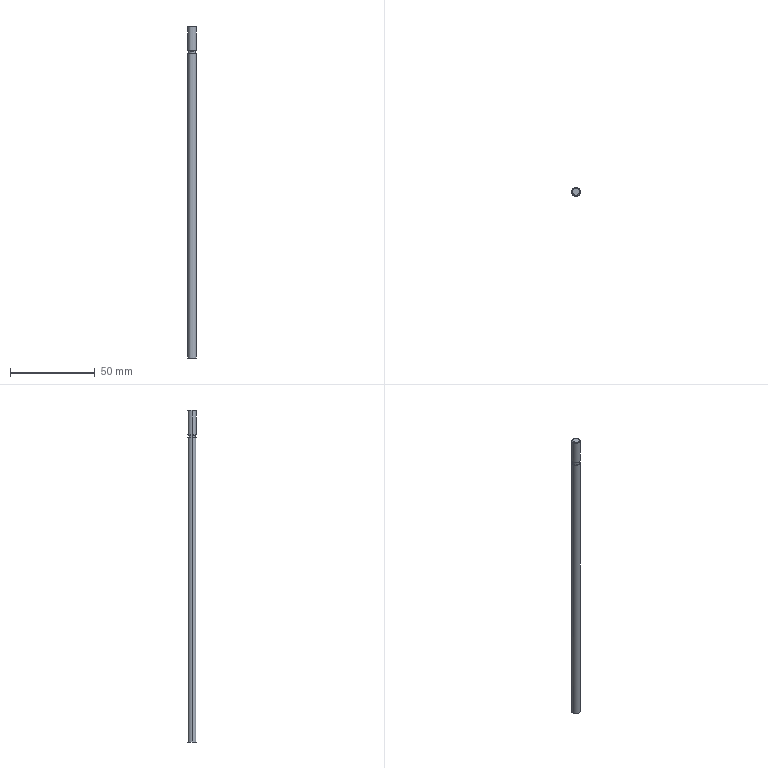Part | NX | features BREP 1 | 1 solid | 13 faces | box 5 x 5 x 196 mm | volume 3835 mm3 | cylinder 6 | cone 4 | plane 3 | commonest cylinder face diameters 5 x4 4.02 x2
STEP:
#1=CARTESIAN_POINT('',(-2.5,0.,3.5));
#2=VERTEX_POINT('',#1);
#3=CARTESIAN_POINT('',(2.5,0.,3.5));
#4=VERTEX_POINT('',#3);
#5=CARTESIAN_POINT('',(0.,0.,3.5));
#6=DIRECTION('',(0.,0.,-1.));
#7=DIRECTION('',(-1.,0.,0.));
#8=AXIS2_PLACEMENT_3D('',#5,#6,#7);
#9=CIRCLE('',#8,2.5);
#10=EDGE_CURVE('',#2,#4,#9,.T.);
#11=ORIENTED_EDGE('',*,*,#10,.T.);
#12=CARTESIAN_POINT('',(2.5,0.,-176.));
#13=VERTEX_POINT('',#12);
#14=CARTESIAN_POINT('',(2.5,0.,-86.25));
#15=DIRECTION('',(0.,0.,-1.));
#16=VECTOR('',#15,1000.);
#17=LINE('',#14,#16);
#18=EDGE_CURVE('',#4,#13,#17,.T.);
#19=ORIENTED_EDGE('',*,*,#18,.T.);
#20=CARTESIAN_POINT('',(-2.5,0.,-176.));
#21=VERTEX_POINT('',#20);
#22=CARTESIAN_POINT('',(0.,0.,-176.));
#23=DIRECTION('',(0.,0.,1.));
#24=DIRECTION('',(-1.,0.,0.));
#25=AXIS2_PLACEMENT_3D('',#22,#23,#24);
#26=CIRCLE('',#25,2.5);
#27=EDGE_CURVE('',#13,#21,#26,.T.);
#28=ORIENTED_EDGE('',*,*,#27,.T.);
#29=CARTESIAN_POINT('',(-2.5,0.,-86.25));
#30=DIRECTION('',(0.,0.,-1.));
#31=VECTOR('',#30,1000.);
#32=LINE('',#29,#31);
#33=EDGE_CURVE('',#2,#21,#32,.T.);
#34=ORIENTED_EDGE('',*,*,#33,.F.);
#35=EDGE_LOOP('',(#11,#19,#28,#34));
#36=FACE_BOUND('',#35,.T.);
#37=CARTESIAN_POINT('',(0.,0.,-86.25));
#38=DIRECTION('',(0.,0.,-1.));
#39=DIRECTION('',(-1.,0.,0.));
#40=AXIS2_PLACEMENT_3D('',#37,#38,#39);
#41=CYLINDRICAL_SURFACE('',#40,2.5);
#42=ADVANCED_FACE('',(#36),#41,.T.);
#43=CARTESIAN_POINT('',(-2.01,0.,5.));
#44=VERTEX_POINT('',#43);
#45=CARTESIAN_POINT('',(2.01,0.,5.));
#46=VERTEX_POINT('',#45);
#47=CARTESIAN_POINT('',(0.,0.,5.));
#48=DIRECTION('',(0.,0.,-1.));
#49=DIRECTION('',(-1.,0.,0.));
#50=AXIS2_PLACEMENT_3D('',#47,#48,#49);
#51=CIRCLE('',#50,2.01);
#52=EDGE_CURVE('',#44,#46,#51,.T.);
#53=ORIENTED_EDGE('',*,*,#52,.T.);
#54=CARTESIAN_POINT('',(2.01,0.,3.5));
#55=VERTEX_POINT('',#54);
#56=CARTESIAN_POINT('',(2.01,0.,4.25));
#57=DIRECTION('',(0.,0.,-1.));
#58=VECTOR('',#57,1000.);
#59=LINE('',#56,#58);
#60=EDGE_CURVE('',#46,#55,#59,.T.);
#61=ORIENTED_EDGE('',*,*,#60,.T.);
#62=CARTESIAN_POINT('',(-2.01,0.,3.5));
#63=VERTEX_POINT('',#62);
#64=CARTESIAN_POINT('',(0.,0.,3.5));
#65=DIRECTION('',(0.,0.,-1.));
#66=DIRECTION('',(-1.,0.,0.));
#67=AXIS2_PLACEMENT_3D('',#64,#65,#66);
#68=CIRCLE('',#67,2.01);
#69=EDGE_CURVE('',#63,#55,#68,.T.);
#70=ORIENTED_EDGE('',*,*,#69,.F.);
#71=CARTESIAN_POINT('',(-2.01,0.,4.25));
#72=DIRECTION('',(0.,0.,-1.));
#73=VECTOR('',#72,1000.);
#74=LINE('',#71,#73);
#75=EDGE_CURVE('',#44,#63,#74,.T.);
#76=ORIENTED_EDGE('',*,*,#75,.F.);
#77=EDGE_LOOP('',(#53,#61,#70,#76));
#78=FACE_BOUND('',#77,.T.);
#79=CARTESIAN_POINT('',(0.,0.,4.25));
#80=DIRECTION('',(0.,0.,-1.));
#81=DIRECTION('',(-1.,0.,0.));
#82=AXIS2_PLACEMENT_3D('',#79,#80,#81);
#83=CYLINDRICAL_SURFACE('',#82,2.01);
#84=ADVANCED_FACE('',(#78),#83,.T.);
#85=ORIENTED_EDGE('',*,*,#52,.F.);
#86=CARTESIAN_POINT('',(-2.5,0.,5.49));
#87=VERTEX_POINT('',#86);
#88=CARTESIAN_POINT('',(-2.5,0.,5.49));
#89=DIRECTION('',(-0.7071,0.,0.7071));
#90=VECTOR('',#89,1000.);
#91=LINE('',#88,#90);
#92=EDGE_CURVE('',#87,#44,#91,.F.);
#93=ORIENTED_EDGE('',*,*,#92,.F.);
#94=CARTESIAN_POINT('',(2.5,0.,5.49));
#95=VERTEX_POINT('',#94);
#96=CARTESIAN_POINT('',(0.,0.,5.49));
#97=DIRECTION('',(0.,0.,-1.));
#98=DIRECTION('',(0.,1.,0.));
#99=AXIS2_PLACEMENT_3D('',#96,#97,#98);
#100=CIRCLE('',#99,2.5);
#101=EDGE_CURVE('',#87,#95,#100,.T.);
#102=ORIENTED_EDGE('',*,*,#101,.T.);
#103=CARTESIAN_POINT('',(2.5,0.,5.49));
#104=DIRECTION('',(0.7071,0.,0.7071));
#105=VECTOR('',#104,1000.);
#106=LINE('',#103,#105);
#107=EDGE_CURVE('',#95,#46,#106,.F.);
#108=ORIENTED_EDGE('',*,*,#107,.T.);
#109=EDGE_LOOP('',(#85,#93,#102,#108));
#110=FACE_BOUND('',#109,.T.);
#111=CARTESIAN_POINT('',(0.,0.,5.49));
#112=DIRECTION('',(0.,0.,1.));
#113=DIRECTION('',(1.,0.,0.));
#114=AXIS2_PLACEMENT_3D('',#111,#112,#113);
#115=CONICAL_SURFACE('',#114,2.5,0.7854);
#116=ADVANCED_FACE('',(#110),#115,.T.);
#117=CARTESIAN_POINT('',(-2.5,0.,19.51));
#118=VERTEX_POINT('',#117);
#119=CARTESIAN_POINT('',(2.5,0.,19.51));
#120=VERTEX_POINT('',#119);
#121=CARTESIAN_POINT('',(0.,0.,19.51));
#122=DIRECTION('',(0.,0.,-1.));
#123=DIRECTION('',(-1.,0.,0.));
#124=AXIS2_PLACEMENT_3D('',#121,#122,#123);
#125=CIRCLE('',#124,2.5);
#126=EDGE_CURVE('',#118,#120,#125,.T.);
#127=ORIENTED_EDGE('',*,*,#126,.T.);
#128=CARTESIAN_POINT('',(2.5,0.,12.5));
#129=DIRECTION('',(0.,0.,-1.));
#130=VECTOR('',#129,1000.);
#131=LINE('',#128,#130);
#132=EDGE_CURVE('',#120,#95,#131,.T.);
#133=ORIENTED_EDGE('',*,*,#132,.T.);
#134=ORIENTED_EDGE('',*,*,#101,.F.);
#135=CARTESIAN_POINT('',(-2.5,0.,12.5));
#136=DIRECTION('',(0.,0.,-1.));
#137=VECTOR('',#136,1000.);
#138=LINE('',#135,#137);
#139=EDGE_CURVE('',#118,#87,#138,.T.);
#140=ORIENTED_EDGE('',*,*,#139,.F.);
#141=EDGE_LOOP('',(#127,#133,#134,#140));
#142=FACE_BOUND('',#141,.T.);
#143=CARTESIAN_POINT('',(0.,0.,12.5));
#144=DIRECTION('',(0.,0.,-1.));
#145=DIRECTION('',(-1.,0.,0.));
#146=AXIS2_PLACEMENT_3D('',#143,#144,#145);
#147=CYLINDRICAL_SURFACE('',#146,2.5);
#148=ADVANCED_FACE('',(#142),#147,.T.);
#149=CARTESIAN_POINT('',(-2.01,0.,20.));
#150=VERTEX_POINT('',#149);
#151=CARTESIAN_POINT('',(2.01,0.,20.));
#152=VERTEX_POINT('',#151);
#153=CARTESIAN_POINT('',(0.,0.,20.));
#154=DIRECTION('',(0.,0.,-1.));
#155=DIRECTION('',(-1.,0.,0.));
#156=AXIS2_PLACEMENT_3D('',#153,#154,#155);
#157=CIRCLE('',#156,2.01);
#158=EDGE_CURVE('',#150,#152,#157,.T.);
#159=ORIENTED_EDGE('',*,*,#158,.T.);
#160=CARTESIAN_POINT('',(2.5,0.,19.51));
#161=DIRECTION('',(0.7071,0.,-0.7071));
#162=VECTOR('',#161,1000.);
#163=LINE('',#160,#162);
#164=EDGE_CURVE('',#152,#120,#163,.T.);
#165=ORIENTED_EDGE('',*,*,#164,.T.);
#166=ORIENTED_EDGE('',*,*,#126,.F.);
#167=CARTESIAN_POINT('',(-2.5,0.,19.51));
#168=DIRECTION('',(-0.7071,0.,-0.7071));
#169=VECTOR('',#168,1000.);
#170=LINE('',#167,#169);
#171=EDGE_CURVE('',#150,#118,#170,.T.);
#172=ORIENTED_EDGE('',*,*,#171,.F.);
#173=EDGE_LOOP('',(#159,#165,#166,#172));
#174=FACE_BOUND('',#173,.T.);
#175=CARTESIAN_POINT('',(0.,0.,19.51));
#176=DIRECTION('',(0.,0.,-1.));
#177=DIRECTION('',(-1.,0.,0.));
#178=AXIS2_PLACEMENT_3D('',#175,#176,#177);
#179=CONICAL_SURFACE('',#178,2.5,0.7854);
#180=ADVANCED_FACE('',(#174),#179,.T.);
#181=ORIENTED_EDGE('',*,*,#18,.F.);
#182=CARTESIAN_POINT('',(0.,0.,3.5));
#183=DIRECTION('',(0.,0.,-1.));
#184=DIRECTION('',(-1.,0.,0.));
#185=AXIS2_PLACEMENT_3D('',#182,#183,#184);
#186=CIRCLE('',#185,2.5);
#187=EDGE_CURVE('',#4,#2,#186,.T.);
#188=ORIENTED_EDGE('',*,*,#187,.T.);
#189=ORIENTED_EDGE('',*,*,#33,.T.);
#190=CARTESIAN_POINT('',(0.,0.,-176.));
#191=DIRECTION('',(0.,0.,1.));
#192=DIRECTION('',(-1.,0.,0.));
#193=AXIS2_PLACEMENT_3D('',#190,#191,#192);
#194=CIRCLE('',#193,2.5);
#195=EDGE_CURVE('',#21,#13,#194,.T.);
#196=ORIENTED_EDGE('',*,*,#195,.T.);
#197=EDGE_LOOP('',(#181,#188,#189,#196));
#198=FACE_BOUND('',#197,.T.);
#199=CARTESIAN_POINT('',(0.,0.,-86.25));
#200=DIRECTION('',(0.,0.,-1.));
#201=DIRECTION('',(-1.,0.,0.));
#202=AXIS2_PLACEMENT_3D('',#199,#200,#201);
#203=CYLINDRICAL_SURFACE('',#202,2.5);
#204=ADVANCED_FACE('',(#198),#203,.T.);
#205=ORIENTED_EDGE('',*,*,#10,.F.);
#206=ORIENTED_EDGE('',*,*,#187,.F.);
#207=EDGE_LOOP('',(#205,#206));
#208=FACE_BOUND('',#207,.T.);
#209=ORIENTED_EDGE('',*,*,#69,.T.);
#210=CARTESIAN_POINT('',(0.,0.,3.5));
#211=DIRECTION('',(0.,0.,-1.));
#212=DIRECTION('',(-1.,0.,0.));
#213=AXIS2_PLACEMENT_3D('',#210,#211,#212);
#214=CIRCLE('',#213,2.01);
#215=EDGE_CURVE('',#55,#63,#214,.T.);
#216=ORIENTED_EDGE('',*,*,#215,.T.);
#217=EDGE_LOOP('',(#209,#216));
#218=FACE_BOUND('',#217,.T.);
#219=CARTESIAN_POINT('',(0.,2.255,3.5));
#220=DIRECTION('',(0.,0.,1.));
#221=DIRECTION('',(1.,0.,0.));
#222=AXIS2_PLACEMENT_3D('',#219,#220,#221);
#223=PLANE('',#222);
#224=ADVANCED_FACE('',(#208,#218),#223,.T.);
#225=ORIENTED_EDGE('',*,*,#195,.F.);
#226=ORIENTED_EDGE('',*,*,#27,.F.);
#227=EDGE_LOOP('',(#225,#226));
#228=FACE_BOUND('',#227,.T.);
#229=CARTESIAN_POINT('',(0.,1.25,-176.));
#230=DIRECTION('',(0.,0.,-1.));
#231=DIRECTION('',(0.,-1.,0.));
#232=AXIS2_PLACEMENT_3D('',#229,#230,#231);
#233=PLANE('',#232);
#234=ADVANCED_FACE('',(#228),#233,.T.);
#235=ORIENTED_EDGE('',*,*,#60,.F.);
#236=CARTESIAN_POINT('',(0.,0.,5.));
#237=DIRECTION('',(0.,0.,-1.));
#238=DIRECTION('',(-1.,0.,0.));
#239=AXIS2_PLACEMENT_3D('',#236,#237,#238);
#240=CIRCLE('',#239,2.01);
#241=EDGE_CURVE('',#46,#44,#240,.T.);
#242=ORIENTED_EDGE('',*,*,#241,.T.);
#243=ORIENTED_EDGE('',*,*,#75,.T.);
#244=ORIENTED_EDGE('',*,*,#215,.F.);
#245=EDGE_LOOP('',(#235,#242,#243,#244));
#246=FACE_BOUND('',#245,.T.);
#247=CARTESIAN_POINT('',(0.,0.,4.25));
#248=DIRECTION('',(0.,0.,-1.));
#249=DIRECTION('',(-1.,0.,0.));
#250=AXIS2_PLACEMENT_3D('',#247,#248,#249);
#251=CYLINDRICAL_SURFACE('',#250,2.01);
#252=ADVANCED_FACE('',(#246),#251,.T.);
#253=ORIENTED_EDGE('',*,*,#92,.T.);
#254=ORIENTED_EDGE('',*,*,#241,.F.);
#255=ORIENTED_EDGE('',*,*,#107,.F.);
#256=CARTESIAN_POINT('',(0.,0.,5.49));
#257=DIRECTION('',(0.,0.,-1.));
#258=DIRECTION('',(0.,1.,0.));
#259=AXIS2_PLACEMENT_3D('',#256,#257,#258);
#260=CIRCLE('',#259,2.5);
#261=EDGE_CURVE('',#95,#87,#260,.T.);
#262=ORIENTED_EDGE('',*,*,#261,.T.);
#263=EDGE_LOOP('',(#253,#254,#255,#262));
#264=FACE_BOUND('',#263,.T.);
#265=CARTESIAN_POINT('',(0.,0.,5.49));
#266=DIRECTION('',(0.,0.,1.));
#267=DIRECTION('',(1.,0.,0.));
#268=AXIS2_PLACEMENT_3D('',#265,#266,#267);
#269=CONICAL_SURFACE('',#268,2.5,0.7854);
#270=ADVANCED_FACE('',(#264),#269,.T.);
#271=ORIENTED_EDGE('',*,*,#132,.F.);
#272=CARTESIAN_POINT('',(0.,0.,19.51));
#273=DIRECTION('',(0.,0.,-1.));
#274=DIRECTION('',(-1.,0.,0.));
#275=AXIS2_PLACEMENT_3D('',#272,#273,#274);
#276=CIRCLE('',#275,2.5);
#277=EDGE_CURVE('',#120,#118,#276,.T.);
#278=ORIENTED_EDGE('',*,*,#277,.T.);
#279=ORIENTED_EDGE('',*,*,#139,.T.);
#280=ORIENTED_EDGE('',*,*,#261,.F.);
#281=EDGE_LOOP('',(#271,#278,#279,#280));
#282=FACE_BOUND('',#281,.T.);
#283=CARTESIAN_POINT('',(0.,0.,12.5));
#284=DIRECTION('',(0.,0.,-1.));
#285=DIRECTION('',(-1.,0.,0.));
#286=AXIS2_PLACEMENT_3D('',#283,#284,#285);
#287=CYLINDRICAL_SURFACE('',#286,2.5);
#288=ADVANCED_FACE('',(#282),#287,.T.);
#289=ORIENTED_EDGE('',*,*,#164,.F.);
#290=CARTESIAN_POINT('',(0.,0.,20.));
#291=DIRECTION('',(0.,0.,-1.));
#292=DIRECTION('',(-1.,0.,0.));
#293=AXIS2_PLACEMENT_3D('',#290,#291,#292);
#294=CIRCLE('',#293,2.01);
#295=EDGE_CURVE('',#152,#150,#294,.T.);
#296=ORIENTED_EDGE('',*,*,#295,.T.);
#297=ORIENTED_EDGE('',*,*,#171,.T.);
#298=ORIENTED_EDGE('',*,*,#277,.F.);
#299=EDGE_LOOP('',(#289,#296,#297,#298));
#300=FACE_BOUND('',#299,.T.);
#301=CARTESIAN_POINT('',(0.,0.,19.51));
#302=DIRECTION('',(0.,0.,-1.));
#303=DIRECTION('',(-1.,0.,0.));
#304=AXIS2_PLACEMENT_3D('',#301,#302,#303);
#305=CONICAL_SURFACE('',#304,2.5,0.7854);
#306=ADVANCED_FACE('',(#300),#305,.T.);
#307=ORIENTED_EDGE('',*,*,#158,.F.);
#308=ORIENTED_EDGE('',*,*,#295,.F.);
#309=EDGE_LOOP('',(#307,#308));
#310=FACE_BOUND('',#309,.T.);
#311=CARTESIAN_POINT('',(0.,1.005,20.));
#312=DIRECTION('',(0.,0.,1.));
#313=DIRECTION('',(1.,0.,0.));
#314=AXIS2_PLACEMENT_3D('',#311,#312,#313);
#315=PLANE('',#314);
#316=ADVANCED_FACE('',(#310),#315,.T.);
#317=CLOSED_SHELL('',(#42,#84,#116,#148,#180,#204,#224,#234,#252,#270,#288,#306,#316));
#318=MANIFOLD_SOLID_BREP('',#317);
#319=(LENGTH_UNIT()NAMED_UNIT(*)SI_UNIT(.MILLI.,.METRE.));
#320=UNCERTAINTY_MEASURE_WITH_UNIT(LENGTH_MEASURE(0.00001),#319,'','');
#321=(NAMED_UNIT(*)PLANE_ANGLE_UNIT()SI_UNIT($,.RADIAN.));
#322=(NAMED_UNIT(*)SI_UNIT($,.STERADIAN.)SOLID_ANGLE_UNIT());
#323=(GEOMETRIC_REPRESENTATION_CONTEXT(3)GLOBAL_UNCERTAINTY_ASSIGNED_CONTEXT((#320))GLOBAL_UNIT_ASSIGNED_CONTEXT((#319,#321,#322))REPRESENTATION_CONTEXT('',''));
#324=ADVANCED_BREP_SHAPE_REPRESENTATION('',(#318),#323);